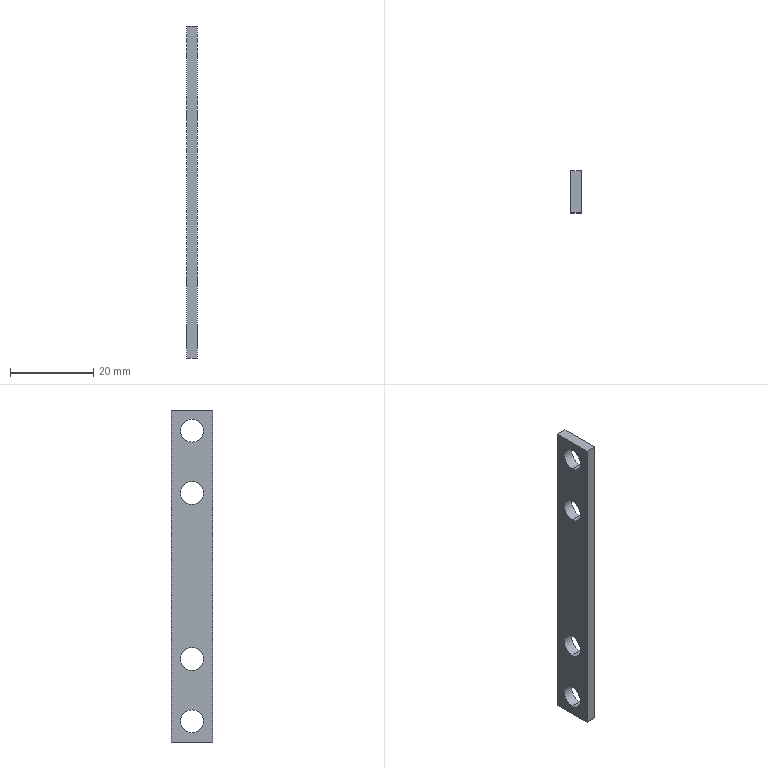Part | SolidWorks | features BaseBody 1 | 1 solid | 14 faces | box 2.5 x 10 x 80 mm | volume 1762 mm3 | cylinder 8 | plane 6 | commonest cylinder face diameters 5.5 x8
STEP:
#1=CARTESIAN_POINT('',(901.946,-4365.973,912.221));
#2=VERTEX_POINT('',#1);
#3=CARTESIAN_POINT('',(901.946,-4365.973,917.721));
#4=VERTEX_POINT('',#3);
#5=CARTESIAN_POINT('',(901.946,-4365.973,914.971));
#6=DIRECTION('',(-1.,0.,0.));
#7=DIRECTION('',(0.,0.,1.));
#8=AXIS2_PLACEMENT_3D('',#5,#6,#7);
#9=CIRCLE('',#8,2.75);
#10=EDGE_CURVE('',#2,#4,#9,.T.);
#11=ORIENTED_EDGE('',*,*,#10,.F.);
#12=CARTESIAN_POINT('',(899.446,-4365.973,912.221));
#13=VERTEX_POINT('',#12);
#14=CARTESIAN_POINT('',(961.392,-4365.973,912.221));
#15=DIRECTION('',(-1.,0.,0.));
#16=VECTOR('',#15,1000.);
#17=LINE('',#14,#16);
#18=EDGE_CURVE('',#2,#13,#17,.T.);
#19=ORIENTED_EDGE('',*,*,#18,.T.);
#20=CARTESIAN_POINT('',(899.446,-4365.973,917.721));
#21=VERTEX_POINT('',#20);
#22=CARTESIAN_POINT('',(899.446,-4365.973,914.971));
#23=DIRECTION('',(1.,0.,0.));
#24=DIRECTION('',(0.,0.,1.));
#25=AXIS2_PLACEMENT_3D('',#22,#23,#24);
#26=CIRCLE('',#25,2.75);
#27=EDGE_CURVE('',#21,#13,#26,.T.);
#28=ORIENTED_EDGE('',*,*,#27,.F.);
#29=CARTESIAN_POINT('',(961.392,-4365.973,917.721));
#30=DIRECTION('',(-1.,0.,0.));
#31=VECTOR('',#30,1000.);
#32=LINE('',#29,#31);
#33=EDGE_CURVE('',#4,#21,#32,.T.);
#34=ORIENTED_EDGE('',*,*,#33,.F.);
#35=EDGE_LOOP('',(#11,#19,#28,#34));
#36=FACE_OUTER_BOUND('',#35,.T.);
#37=CARTESIAN_POINT('',(961.392,-4365.973,914.971));
#38=DIRECTION('',(-1.,0.,0.));
#39=DIRECTION('',(0.,0.,1.));
#40=AXIS2_PLACEMENT_3D('',#37,#38,#39);
#41=CYLINDRICAL_SURFACE('',#40,2.75);
#42=ADVANCED_FACE('',(#36),#41,.F.);
#43=CARTESIAN_POINT('',(899.446,-4365.973,877.721));
#44=VERTEX_POINT('',#43);
#45=CARTESIAN_POINT('',(899.446,-4365.973,872.221));
#46=VERTEX_POINT('',#45);
#47=CARTESIAN_POINT('',(899.446,-4365.973,874.971));
#48=DIRECTION('',(1.,0.,0.));
#49=DIRECTION('',(0.,0.,-1.));
#50=AXIS2_PLACEMENT_3D('',#47,#48,#49);
#51=CIRCLE('',#50,2.75);
#52=EDGE_CURVE('',#44,#46,#51,.T.);
#53=ORIENTED_EDGE('',*,*,#52,.F.);
#54=CARTESIAN_POINT('',(901.946,-4365.973,877.721));
#55=VERTEX_POINT('',#54);
#56=CARTESIAN_POINT('',(961.392,-4365.973,877.721));
#57=DIRECTION('',(1.,0.,0.));
#58=VECTOR('',#57,1000.);
#59=LINE('',#56,#58);
#60=EDGE_CURVE('',#44,#55,#59,.T.);
#61=ORIENTED_EDGE('',*,*,#60,.T.);
#62=CARTESIAN_POINT('',(901.946,-4365.973,872.221));
#63=VERTEX_POINT('',#62);
#64=CARTESIAN_POINT('',(901.946,-4365.973,874.971));
#65=DIRECTION('',(-1.,0.,0.));
#66=DIRECTION('',(0.,0.,-1.));
#67=AXIS2_PLACEMENT_3D('',#64,#65,#66);
#68=CIRCLE('',#67,2.75);
#69=EDGE_CURVE('',#63,#55,#68,.T.);
#70=ORIENTED_EDGE('',*,*,#69,.F.);
#71=CARTESIAN_POINT('',(961.392,-4365.973,872.221));
#72=DIRECTION('',(1.,0.,0.));
#73=VECTOR('',#72,1000.);
#74=LINE('',#71,#73);
#75=EDGE_CURVE('',#46,#63,#74,.T.);
#76=ORIENTED_EDGE('',*,*,#75,.F.);
#77=EDGE_LOOP('',(#53,#61,#70,#76));
#78=FACE_OUTER_BOUND('',#77,.T.);
#79=CARTESIAN_POINT('',(961.392,-4365.973,874.971));
#80=DIRECTION('',(1.,0.,0.));
#81=DIRECTION('',(0.,0.,-1.));
#82=AXIS2_PLACEMENT_3D('',#79,#80,#81);
#83=CYLINDRICAL_SURFACE('',#82,2.75);
#84=ADVANCED_FACE('',(#78),#83,.F.);
#85=CARTESIAN_POINT('',(899.446,-4365.973,862.721));
#86=VERTEX_POINT('',#85);
#87=CARTESIAN_POINT('',(899.446,-4365.973,857.221));
#88=VERTEX_POINT('',#87);
#89=CARTESIAN_POINT('',(899.446,-4365.973,859.971));
#90=DIRECTION('',(1.,0.,0.));
#91=DIRECTION('',(0.,0.,-1.));
#92=AXIS2_PLACEMENT_3D('',#89,#90,#91);
#93=CIRCLE('',#92,2.75);
#94=EDGE_CURVE('',#86,#88,#93,.T.);
#95=ORIENTED_EDGE('',*,*,#94,.F.);
#96=CARTESIAN_POINT('',(901.946,-4365.973,862.721));
#97=VERTEX_POINT('',#96);
#98=CARTESIAN_POINT('',(961.392,-4365.973,862.721));
#99=DIRECTION('',(1.,0.,0.));
#100=VECTOR('',#99,1000.);
#101=LINE('',#98,#100);
#102=EDGE_CURVE('',#86,#97,#101,.T.);
#103=ORIENTED_EDGE('',*,*,#102,.T.);
#104=CARTESIAN_POINT('',(901.946,-4365.973,857.221));
#105=VERTEX_POINT('',#104);
#106=CARTESIAN_POINT('',(901.946,-4365.973,859.971));
#107=DIRECTION('',(-1.,0.,0.));
#108=DIRECTION('',(0.,0.,-1.));
#109=AXIS2_PLACEMENT_3D('',#106,#107,#108);
#110=CIRCLE('',#109,2.75);
#111=EDGE_CURVE('',#105,#97,#110,.T.);
#112=ORIENTED_EDGE('',*,*,#111,.F.);
#113=CARTESIAN_POINT('',(961.392,-4365.973,857.221));
#114=DIRECTION('',(1.,0.,0.));
#115=VECTOR('',#114,1000.);
#116=LINE('',#113,#115);
#117=EDGE_CURVE('',#88,#105,#116,.T.);
#118=ORIENTED_EDGE('',*,*,#117,.F.);
#119=EDGE_LOOP('',(#95,#103,#112,#118));
#120=FACE_OUTER_BOUND('',#119,.T.);
#121=CARTESIAN_POINT('',(961.392,-4365.973,859.971));
#122=DIRECTION('',(1.,0.,0.));
#123=DIRECTION('',(0.,0.,-1.));
#124=AXIS2_PLACEMENT_3D('',#121,#122,#123);
#125=CYLINDRICAL_SURFACE('',#124,2.75);
#126=ADVANCED_FACE('',(#120),#125,.F.);
#127=CARTESIAN_POINT('',(901.946,-4365.973,927.221));
#128=VERTEX_POINT('',#127);
#129=CARTESIAN_POINT('',(901.946,-4365.973,932.721));
#130=VERTEX_POINT('',#129);
#131=CARTESIAN_POINT('',(901.946,-4365.973,929.971));
#132=DIRECTION('',(-1.,0.,0.));
#133=DIRECTION('',(0.,0.,1.));
#134=AXIS2_PLACEMENT_3D('',#131,#132,#133);
#135=CIRCLE('',#134,2.75);
#136=EDGE_CURVE('',#128,#130,#135,.T.);
#137=ORIENTED_EDGE('',*,*,#136,.F.);
#138=CARTESIAN_POINT('',(899.446,-4365.973,927.221));
#139=VERTEX_POINT('',#138);
#140=CARTESIAN_POINT('',(961.392,-4365.973,927.221));
#141=DIRECTION('',(-1.,0.,0.));
#142=VECTOR('',#141,1000.);
#143=LINE('',#140,#142);
#144=EDGE_CURVE('',#128,#139,#143,.T.);
#145=ORIENTED_EDGE('',*,*,#144,.T.);
#146=CARTESIAN_POINT('',(899.446,-4365.973,932.721));
#147=VERTEX_POINT('',#146);
#148=CARTESIAN_POINT('',(899.446,-4365.973,929.971));
#149=DIRECTION('',(1.,0.,0.));
#150=DIRECTION('',(0.,0.,1.));
#151=AXIS2_PLACEMENT_3D('',#148,#149,#150);
#152=CIRCLE('',#151,2.75);
#153=EDGE_CURVE('',#147,#139,#152,.T.);
#154=ORIENTED_EDGE('',*,*,#153,.F.);
#155=CARTESIAN_POINT('',(961.392,-4365.973,932.721));
#156=DIRECTION('',(-1.,0.,0.));
#157=VECTOR('',#156,1000.);
#158=LINE('',#155,#157);
#159=EDGE_CURVE('',#130,#147,#158,.T.);
#160=ORIENTED_EDGE('',*,*,#159,.F.);
#161=EDGE_LOOP('',(#137,#145,#154,#160));
#162=FACE_OUTER_BOUND('',#161,.T.);
#163=CARTESIAN_POINT('',(961.392,-4365.973,929.971));
#164=DIRECTION('',(-1.,0.,0.));
#165=DIRECTION('',(0.,0.,1.));
#166=AXIS2_PLACEMENT_3D('',#163,#164,#165);
#167=CYLINDRICAL_SURFACE('',#166,2.75);
#168=ADVANCED_FACE('',(#162),#167,.F.);
#169=CARTESIAN_POINT('',(899.446,-4360.973,854.971));
#170=VERTEX_POINT('',#169);
#171=CARTESIAN_POINT('',(899.446,-4370.973,854.971));
#172=VERTEX_POINT('',#171);
#173=CARTESIAN_POINT('',(899.446,-4360.973,854.971));
#174=DIRECTION('',(0.,-1.,0.));
#175=VECTOR('',#174,1000.);
#176=LINE('',#173,#175);
#177=EDGE_CURVE('',#170,#172,#176,.T.);
#178=ORIENTED_EDGE('',*,*,#177,.T.);
#179=CARTESIAN_POINT('',(899.446,-4370.973,934.971));
#180=VERTEX_POINT('',#179);
#181=CARTESIAN_POINT('',(899.446,-4370.973,854.971));
#182=DIRECTION('',(0.,0.,1.));
#183=VECTOR('',#182,1000.);
#184=LINE('',#181,#183);
#185=EDGE_CURVE('',#172,#180,#184,.T.);
#186=ORIENTED_EDGE('',*,*,#185,.T.);
#187=CARTESIAN_POINT('',(899.446,-4360.973,934.971));
#188=VERTEX_POINT('',#187);
#189=CARTESIAN_POINT('',(899.446,-4360.973,934.971));
#190=DIRECTION('',(0.,1.,0.));
#191=VECTOR('',#190,1000.);
#192=LINE('',#189,#191);
#193=EDGE_CURVE('',#180,#188,#192,.T.);
#194=ORIENTED_EDGE('',*,*,#193,.T.);
#195=CARTESIAN_POINT('',(899.446,-4360.973,854.971));
#196=DIRECTION('',(0.,0.,-1.));
#197=VECTOR('',#196,1000.);
#198=LINE('',#195,#197);
#199=EDGE_CURVE('',#188,#170,#198,.T.);
#200=ORIENTED_EDGE('',*,*,#199,.T.);
#201=EDGE_LOOP('',(#178,#186,#194,#200));
#202=FACE_OUTER_BOUND('',#201,.T.);
#203=ORIENTED_EDGE('',*,*,#27,.T.);
#204=CARTESIAN_POINT('',(899.446,-4365.973,914.971));
#205=DIRECTION('',(1.,0.,0.));
#206=DIRECTION('',(0.,0.,1.));
#207=AXIS2_PLACEMENT_3D('',#204,#205,#206);
#208=CIRCLE('',#207,2.75);
#209=EDGE_CURVE('',#13,#21,#208,.T.);
#210=ORIENTED_EDGE('',*,*,#209,.T.);
#211=EDGE_LOOP('',(#203,#210));
#212=FACE_BOUND('',#211,.T.);
#213=CARTESIAN_POINT('',(899.446,-4365.973,874.971));
#214=DIRECTION('',(1.,0.,0.));
#215=DIRECTION('',(0.,0.,-1.));
#216=AXIS2_PLACEMENT_3D('',#213,#214,#215);
#217=CIRCLE('',#216,2.75);
#218=EDGE_CURVE('',#46,#44,#217,.T.);
#219=ORIENTED_EDGE('',*,*,#218,.T.);
#220=ORIENTED_EDGE('',*,*,#52,.T.);
#221=EDGE_LOOP('',(#219,#220));
#222=FACE_BOUND('',#221,.T.);
#223=CARTESIAN_POINT('',(899.446,-4365.973,859.971));
#224=DIRECTION('',(1.,0.,0.));
#225=DIRECTION('',(0.,0.,-1.));
#226=AXIS2_PLACEMENT_3D('',#223,#224,#225);
#227=CIRCLE('',#226,2.75);
#228=EDGE_CURVE('',#88,#86,#227,.T.);
#229=ORIENTED_EDGE('',*,*,#228,.T.);
#230=ORIENTED_EDGE('',*,*,#94,.T.);
#231=EDGE_LOOP('',(#229,#230));
#232=FACE_BOUND('',#231,.T.);
#233=ORIENTED_EDGE('',*,*,#153,.T.);
#234=CARTESIAN_POINT('',(899.446,-4365.973,929.971));
#235=DIRECTION('',(1.,0.,0.));
#236=DIRECTION('',(0.,0.,1.));
#237=AXIS2_PLACEMENT_3D('',#234,#235,#236);
#238=CIRCLE('',#237,2.75);
#239=EDGE_CURVE('',#139,#147,#238,.T.);
#240=ORIENTED_EDGE('',*,*,#239,.T.);
#241=EDGE_LOOP('',(#233,#240));
#242=FACE_BOUND('',#241,.T.);
#243=CARTESIAN_POINT('',(899.446,-4360.973,854.971));
#244=DIRECTION('',(-1.,0.,0.));
#245=DIRECTION('',(0.,0.,1.));
#246=AXIS2_PLACEMENT_3D('',#243,#244,#245);
#247=PLANE('',#246);
#248=ADVANCED_FACE('',(#202,#212,#222,#232,#242),#247,.T.);
#249=CARTESIAN_POINT('',(901.946,-4370.973,854.971));
#250=VERTEX_POINT('',#249);
#251=CARTESIAN_POINT('',(899.446,-4370.973,854.971));
#252=DIRECTION('',(1.,0.,0.));
#253=VECTOR('',#252,1000.);
#254=LINE('',#251,#253);
#255=EDGE_CURVE('',#172,#250,#254,.T.);
#256=ORIENTED_EDGE('',*,*,#255,.T.);
#257=CARTESIAN_POINT('',(901.946,-4370.973,934.971));
#258=VERTEX_POINT('',#257);
#259=CARTESIAN_POINT('',(901.946,-4370.973,854.971));
#260=DIRECTION('',(0.,0.,1.));
#261=VECTOR('',#260,1000.);
#262=LINE('',#259,#261);
#263=EDGE_CURVE('',#250,#258,#262,.T.);
#264=ORIENTED_EDGE('',*,*,#263,.T.);
#265=CARTESIAN_POINT('',(899.446,-4370.973,934.971));
#266=DIRECTION('',(-1.,0.,0.));
#267=VECTOR('',#266,1000.);
#268=LINE('',#265,#267);
#269=EDGE_CURVE('',#258,#180,#268,.T.);
#270=ORIENTED_EDGE('',*,*,#269,.T.);
#271=ORIENTED_EDGE('',*,*,#185,.F.);
#272=EDGE_LOOP('',(#256,#264,#270,#271));
#273=FACE_OUTER_BOUND('',#272,.T.);
#274=CARTESIAN_POINT('',(899.446,-4370.973,854.971));
#275=DIRECTION('',(0.,-1.,0.));
#276=DIRECTION('',(0.,0.,-1.));
#277=AXIS2_PLACEMENT_3D('',#274,#275,#276);
#278=PLANE('',#277);
#279=ADVANCED_FACE('',(#273),#278,.T.);
#280=ORIENTED_EDGE('',*,*,#177,.F.);
#281=CARTESIAN_POINT('',(901.946,-4360.973,854.971));
#282=VERTEX_POINT('',#281);
#283=CARTESIAN_POINT('',(900.696,-4360.973,854.971));
#284=DIRECTION('',(-1.,0.,0.));
#285=VECTOR('',#284,1000.);
#286=LINE('',#283,#285);
#287=EDGE_CURVE('',#282,#170,#286,.T.);
#288=ORIENTED_EDGE('',*,*,#287,.F.);
#289=CARTESIAN_POINT('',(901.946,-4365.973,854.971));
#290=DIRECTION('',(0.,1.,0.));
#291=VECTOR('',#290,1000.);
#292=LINE('',#289,#291);
#293=EDGE_CURVE('',#250,#282,#292,.T.);
#294=ORIENTED_EDGE('',*,*,#293,.F.);
#295=ORIENTED_EDGE('',*,*,#255,.F.);
#296=EDGE_LOOP('',(#280,#288,#294,#295));
#297=FACE_OUTER_BOUND('',#296,.T.);
#298=CARTESIAN_POINT('',(900.696,-4365.973,854.971));
#299=DIRECTION('',(0.,0.,1.));
#300=DIRECTION('',(1.,0.,0.));
#301=AXIS2_PLACEMENT_3D('',#298,#299,#300);
#302=PLANE('',#301);
#303=ADVANCED_FACE('',(#297),#302,.F.);
#304=ORIENTED_EDGE('',*,*,#287,.T.);
#305=ORIENTED_EDGE('',*,*,#199,.F.);
#306=CARTESIAN_POINT('',(901.946,-4360.973,934.971));
#307=VERTEX_POINT('',#306);
#308=CARTESIAN_POINT('',(901.946,-4360.973,934.971));
#309=DIRECTION('',(1.,0.,0.));
#310=VECTOR('',#309,1000.);
#311=LINE('',#308,#310);
#312=EDGE_CURVE('',#188,#307,#311,.T.);
#313=ORIENTED_EDGE('',*,*,#312,.T.);
#314=CARTESIAN_POINT('',(901.946,-4360.973,854.971));
#315=DIRECTION('',(0.,0.,-1.));
#316=VECTOR('',#315,1000.);
#317=LINE('',#314,#316);
#318=EDGE_CURVE('',#307,#282,#317,.T.);
#319=ORIENTED_EDGE('',*,*,#318,.T.);
#320=EDGE_LOOP('',(#304,#305,#313,#319));
#321=FACE_OUTER_BOUND('',#320,.T.);
#322=CARTESIAN_POINT('',(901.946,-4360.973,854.971));
#323=DIRECTION('',(0.,1.,0.));
#324=DIRECTION('',(0.,0.,1.));
#325=AXIS2_PLACEMENT_3D('',#322,#323,#324);
#326=PLANE('',#325);
#327=ADVANCED_FACE('',(#321),#326,.T.);
#328=ORIENTED_EDGE('',*,*,#193,.F.);
#329=ORIENTED_EDGE('',*,*,#269,.F.);
#330=CARTESIAN_POINT('',(901.946,-4365.973,934.971));
#331=DIRECTION('',(0.,1.,0.));
#332=VECTOR('',#331,1000.);
#333=LINE('',#330,#332);
#334=EDGE_CURVE('',#258,#307,#333,.T.);
#335=ORIENTED_EDGE('',*,*,#334,.T.);
#336=ORIENTED_EDGE('',*,*,#312,.F.);
#337=EDGE_LOOP('',(#328,#329,#335,#336));
#338=FACE_OUTER_BOUND('',#337,.T.);
#339=CARTESIAN_POINT('',(900.696,-4365.973,934.971));
#340=DIRECTION('',(0.,0.,1.));
#341=DIRECTION('',(1.,0.,0.));
#342=AXIS2_PLACEMENT_3D('',#339,#340,#341);
#343=PLANE('',#342);
#344=ADVANCED_FACE('',(#338),#343,.T.);
#345=ORIENTED_EDGE('',*,*,#18,.F.);
#346=CARTESIAN_POINT('',(901.946,-4365.973,914.971));
#347=DIRECTION('',(-1.,0.,0.));
#348=DIRECTION('',(0.,0.,1.));
#349=AXIS2_PLACEMENT_3D('',#346,#347,#348);
#350=CIRCLE('',#349,2.75);
#351=EDGE_CURVE('',#4,#2,#350,.T.);
#352=ORIENTED_EDGE('',*,*,#351,.F.);
#353=ORIENTED_EDGE('',*,*,#33,.T.);
#354=ORIENTED_EDGE('',*,*,#209,.F.);
#355=EDGE_LOOP('',(#345,#352,#353,#354));
#356=FACE_OUTER_BOUND('',#355,.T.);
#357=CARTESIAN_POINT('',(961.392,-4365.973,914.971));
#358=DIRECTION('',(-1.,0.,0.));
#359=DIRECTION('',(0.,0.,1.));
#360=AXIS2_PLACEMENT_3D('',#357,#358,#359);
#361=CYLINDRICAL_SURFACE('',#360,2.75);
#362=ADVANCED_FACE('',(#356),#361,.F.);
#363=ORIENTED_EDGE('',*,*,#60,.F.);
#364=ORIENTED_EDGE('',*,*,#218,.F.);
#365=ORIENTED_EDGE('',*,*,#75,.T.);
#366=CARTESIAN_POINT('',(901.946,-4365.973,874.971));
#367=DIRECTION('',(-1.,0.,0.));
#368=DIRECTION('',(0.,0.,-1.));
#369=AXIS2_PLACEMENT_3D('',#366,#367,#368);
#370=CIRCLE('',#369,2.75);
#371=EDGE_CURVE('',#55,#63,#370,.T.);
#372=ORIENTED_EDGE('',*,*,#371,.F.);
#373=EDGE_LOOP('',(#363,#364,#365,#372));
#374=FACE_OUTER_BOUND('',#373,.T.);
#375=CARTESIAN_POINT('',(961.392,-4365.973,874.971));
#376=DIRECTION('',(1.,0.,0.));
#377=DIRECTION('',(0.,0.,-1.));
#378=AXIS2_PLACEMENT_3D('',#375,#376,#377);
#379=CYLINDRICAL_SURFACE('',#378,2.75);
#380=ADVANCED_FACE('',(#374),#379,.F.);
#381=ORIENTED_EDGE('',*,*,#102,.F.);
#382=ORIENTED_EDGE('',*,*,#228,.F.);
#383=ORIENTED_EDGE('',*,*,#117,.T.);
#384=CARTESIAN_POINT('',(901.946,-4365.973,859.971));
#385=DIRECTION('',(-1.,0.,0.));
#386=DIRECTION('',(0.,0.,-1.));
#387=AXIS2_PLACEMENT_3D('',#384,#385,#386);
#388=CIRCLE('',#387,2.75);
#389=EDGE_CURVE('',#97,#105,#388,.T.);
#390=ORIENTED_EDGE('',*,*,#389,.F.);
#391=EDGE_LOOP('',(#381,#382,#383,#390));
#392=FACE_OUTER_BOUND('',#391,.T.);
#393=CARTESIAN_POINT('',(961.392,-4365.973,859.971));
#394=DIRECTION('',(1.,0.,0.));
#395=DIRECTION('',(0.,0.,-1.));
#396=AXIS2_PLACEMENT_3D('',#393,#394,#395);
#397=CYLINDRICAL_SURFACE('',#396,2.75);
#398=ADVANCED_FACE('',(#392),#397,.F.);
#399=ORIENTED_EDGE('',*,*,#144,.F.);
#400=CARTESIAN_POINT('',(901.946,-4365.973,929.971));
#401=DIRECTION('',(-1.,0.,0.));
#402=DIRECTION('',(0.,0.,1.));
#403=AXIS2_PLACEMENT_3D('',#400,#401,#402);
#404=CIRCLE('',#403,2.75);
#405=EDGE_CURVE('',#130,#128,#404,.T.);
#406=ORIENTED_EDGE('',*,*,#405,.F.);
#407=ORIENTED_EDGE('',*,*,#159,.T.);
#408=ORIENTED_EDGE('',*,*,#239,.F.);
#409=EDGE_LOOP('',(#399,#406,#407,#408));
#410=FACE_OUTER_BOUND('',#409,.T.);
#411=CARTESIAN_POINT('',(961.392,-4365.973,929.971));
#412=DIRECTION('',(-1.,0.,0.));
#413=DIRECTION('',(0.,0.,1.));
#414=AXIS2_PLACEMENT_3D('',#411,#412,#413);
#415=CYLINDRICAL_SURFACE('',#414,2.75);
#416=ADVANCED_FACE('',(#410),#415,.F.);
#417=ORIENTED_EDGE('',*,*,#293,.T.);
#418=ORIENTED_EDGE('',*,*,#318,.F.);
#419=ORIENTED_EDGE('',*,*,#334,.F.);
#420=ORIENTED_EDGE('',*,*,#263,.F.);
#421=EDGE_LOOP('',(#417,#418,#419,#420));
#422=FACE_OUTER_BOUND('',#421,.T.);
#423=ORIENTED_EDGE('',*,*,#351,.T.);
#424=ORIENTED_EDGE('',*,*,#10,.T.);
#425=EDGE_LOOP('',(#423,#424));
#426=FACE_BOUND('',#425,.T.);
#427=ORIENTED_EDGE('',*,*,#69,.T.);
#428=ORIENTED_EDGE('',*,*,#371,.T.);
#429=EDGE_LOOP('',(#427,#428));
#430=FACE_BOUND('',#429,.T.);
#431=ORIENTED_EDGE('',*,*,#111,.T.);
#432=ORIENTED_EDGE('',*,*,#389,.T.);
#433=EDGE_LOOP('',(#431,#432));
#434=FACE_BOUND('',#433,.T.);
#435=ORIENTED_EDGE('',*,*,#405,.T.);
#436=ORIENTED_EDGE('',*,*,#136,.T.);
#437=EDGE_LOOP('',(#435,#436));
#438=FACE_BOUND('',#437,.T.);
#439=CARTESIAN_POINT('',(901.946,-4370.973,854.971));
#440=DIRECTION('',(1.,0.,0.));
#441=DIRECTION('',(0.,0.,-1.));
#442=AXIS2_PLACEMENT_3D('',#439,#440,#441);
#443=PLANE('',#442);
#444=ADVANCED_FACE('',(#422,#426,#430,#434,#438),#443,.T.);
#445=CLOSED_SHELL('',(#42,#84,#126,#168,#248,#279,#303,#327,#344,#362,#380,#398,#416,#444));
#446=MANIFOLD_SOLID_BREP('',#445);
#447=CARTESIAN_POINT('',(0.,0.,0.));
#448=DIRECTION('',(0.,0.,1.));
#449=DIRECTION('',(1.,0.,0.));
#450=AXIS2_PLACEMENT_3D('',#447,#448,#449);
#451=(LENGTH_UNIT()NAMED_UNIT(*)SI_UNIT(.MILLI.,.METRE.));
#452=UNCERTAINTY_MEASURE_WITH_UNIT(LENGTH_MEASURE(0.00001),#451,'','');
#453=(NAMED_UNIT(*)PLANE_ANGLE_UNIT()SI_UNIT($,.RADIAN.));
#454=(NAMED_UNIT(*)SI_UNIT($,.STERADIAN.)SOLID_ANGLE_UNIT());
#455=(GEOMETRIC_REPRESENTATION_CONTEXT(3)GLOBAL_UNCERTAINTY_ASSIGNED_CONTEXT((#452))GLOBAL_UNIT_ASSIGNED_CONTEXT((#451,#453,#454))REPRESENTATION_CONTEXT('',''));
#456=ADVANCED_BREP_SHAPE_REPRESENTATION('',(#446,#450),#455);